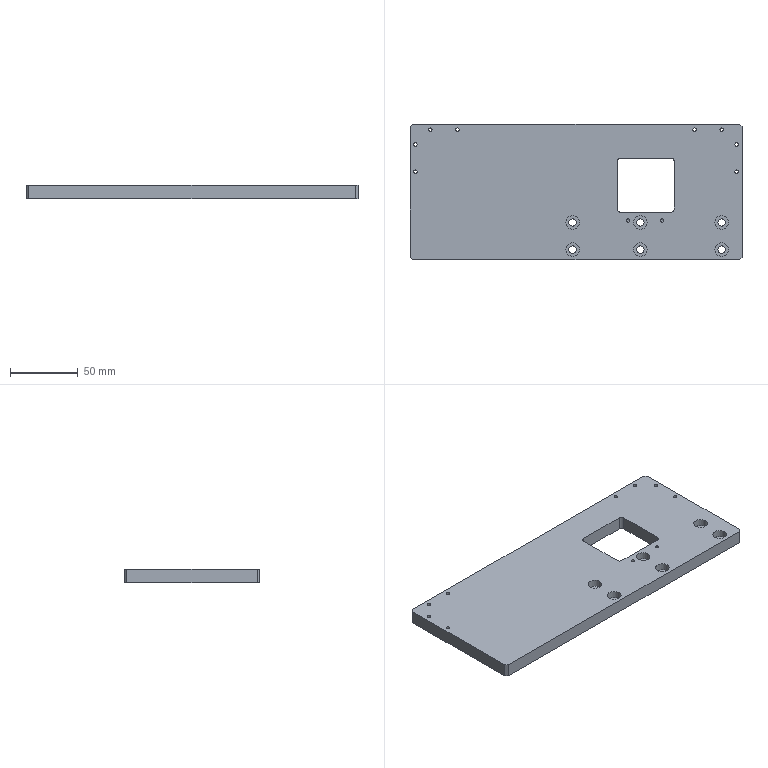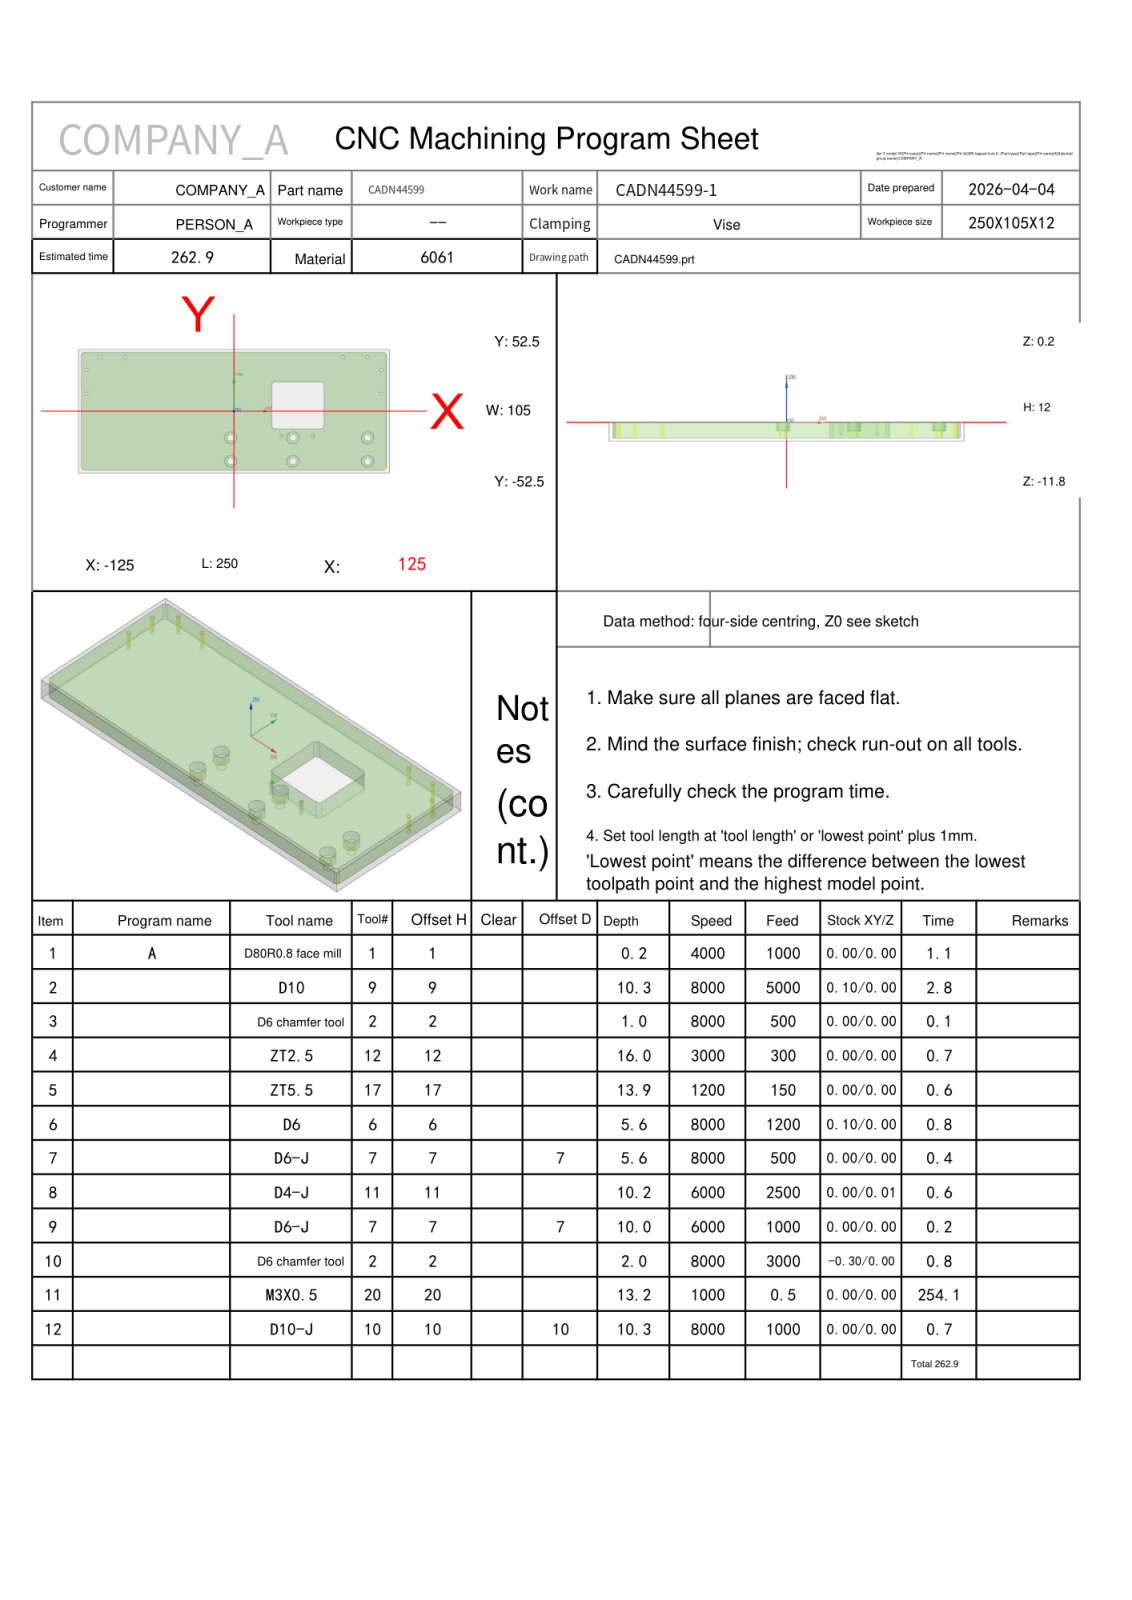NC program | NX | posted by the shop | part box 245 x 100 x 10 mm
Lines 755 to 1778 of 5259:
N8 T11 M06
(D4-J  D=4. R=0. H=11 ce=0.00 di=0.01)
G00 G90 G54 X33.121 Y-9.46 M03 S6000
G43 H11 Z20.
M08
Z.306
G01 X33.114 Y-9.461 Z.22 F2000.
X33.094 Y-9.463 Z.142
X33.064 Y-9.468 Z.072
X33.024 Y-9.475 Z.01
X32.977 Y-9.485 Z-.046
X32.925 Y-9.498 Z-.095
X32.868 Y-9.514 Z-.137
X32.811 Y-9.533 Z-.174
X32.753 Y-9.557 Z-.205
X32.696 Y-9.584 Z-.231
X32.644 Y-9.615 Z-.252
X32.597 Y-9.652 Z-.268
X32.557 Y-9.692 Z-.28
X32.527 Y-9.738 Z-.288
X32.507 Y-9.79 Z-.293
X32.5 Y-9.847 Z-.294
Y-12.565 F2500.
G03 X32.935 Y-13. I.435 J0.0
G01 X35.653
X35.696 Y-12.984 Z-.295
X35.718 Y-12.938 Z-.298
X35.72 Y-12.866 Z-.302
X35.703 Y-12.772 Z-.307
X35.67 Y-12.657 Z-.314
X35.622 Y-12.527 Z-.322
X35.56 Y-12.384 Z-.331
X35.486 Y-12.232 Z-.341
X35.402 Y-12.074 Z-.351
X35.309 Y-11.913 Z-.362
X35.209 Y-11.754 Z-.374
X34.969 Y-11.417 Z-.4
X34.704 Y-11.103 Z-.427
X34.413 Y-10.812 Z-.455
X34.098 Y-10.545 Z-.482
X33.76 Y-10.303 Z-.509
X33.599 Y-10.202 Z-.52
X33.437 Y-10.108 Z-.531
X33.278 Y-10.022 Z-.542
X33.124 Y-9.947 Z-.551
X32.979 Y-9.883 Z-.56
X32.847 Y-9.834 Z-.568
X32.731 Y-9.799 Z-.575
X32.635 Y-9.782 Z-.581
X32.563 Y-9.783 Z-.585
X32.516 Y-9.804 Z-.587
X32.5 Y-9.847 Z-.588
Y-12.565
G03 X32.935 Y-13. I.435 J0.0
G01 X35.653
X35.696 Y-12.984 Z-.589
X35.718 Y-12.938 Z-.592
X35.72 Y-12.866 Z-.596
X35.703 Y-12.772 Z-.601
X35.67 Y-12.657 Z-.608
X35.622 Y-12.527 Z-.616
X35.56 Y-12.384 Z-.625
X35.486 Y-12.232 Z-.635
X35.402 Y-12.074 Z-.645
X35.309 Y-11.913 Z-.656
X35.209 Y-11.754 Z-.668
X34.969 Y-11.417 Z-.694
X34.704 Y-11.103 Z-.722
X34.413 Y-10.812 Z-.749
X34.098 Y-10.545 Z-.776
X33.76 Y-10.303 Z-.803
X33.599 Y-10.202 Z-.814
X33.437 Y-10.108 Z-.825
X33.278 Y-10.022 Z-.836
X33.124 Y-9.947 Z-.846
X32.979 Y-9.883 Z-.855
X32.847 Y-9.834 Z-.862
X32.731 Y-9.799 Z-.869
X32.635 Y-9.782 Z-.875
X32.563 Y-9.783 Z-.879
X32.516 Y-9.804 Z-.881
X32.5 Y-9.847 Z-.882
Y-12.565
G03 X32.935 Y-13. I.435 J0.0
G01 X35.653
X35.696 Y-12.984 Z-.883
X35.718 Y-12.938 Z-.886
X35.72 Y-12.866 Z-.89
X35.703 Y-12.772 Z-.895
X35.67 Y-12.657 Z-.902
X35.622 Y-12.527 Z-.91
X35.56 Y-12.384 Z-.919
X35.486 Y-12.232 Z-.929
X35.402 Y-12.074 Z-.939
X35.309 Y-11.913 Z-.95
X35.209 Y-11.754 Z-.962
X34.969 Y-11.417 Z-.988
X34.704 Y-11.103 Z-1.016
X34.413 Y-10.812 Z-1.043
X34.098 Y-10.545 Z-1.07
X33.76 Y-10.303 Z-1.097
X33.599 Y-10.202 Z-1.108
X33.437 Y-10.108 Z-1.119
X33.278 Y-10.022 Z-1.13
X33.124 Y-9.947 Z-1.14
X32.979 Y-9.883 Z-1.149
X32.847 Y-9.834 Z-1.157
X32.731 Y-9.799 Z-1.163
X32.635 Y-9.782 Z-1.169
X32.563 Y-9.783 Z-1.173
X32.516 Y-9.804 Z-1.176
X32.5 Y-9.847
Y-12.565
G03 X32.935 Y-13. I.435 J0.0
G01 X35.653
X35.696 Y-12.984 Z-1.177
X35.718 Y-12.938 Z-1.18
X35.72 Y-12.866 Z-1.184
X35.703 Y-12.772 Z-1.19
X35.67 Y-12.657 Z-1.196
X35.622 Y-12.527 Z-1.204
X35.56 Y-12.384 Z-1.213
X35.486 Y-12.232 Z-1.223
X35.402 Y-12.074 Z-1.234
X35.309 Y-11.913 Z-1.245
X35.209 Y-11.754 Z-1.256
X34.969 Y-11.417 Z-1.283
X34.704 Y-11.103 Z-1.31
X34.413 Y-10.812 Z-1.337
X34.098 Y-10.545 Z-1.365
X33.76 Y-10.303 Z-1.391
X33.599 Y-10.202 Z-1.402
X33.437 Y-10.108 Z-1.414
X33.278 Y-10.022 Z-1.424
X33.124 Y-9.947 Z-1.434
X32.979 Y-9.883 Z-1.443
X32.847 Y-9.834 Z-1.451
X32.731 Y-9.799 Z-1.457
X32.635 Y-9.782 Z-1.463
X32.563 Y-9.783 Z-1.467
X32.516 Y-9.804 Z-1.47
X32.5 Y-9.847 Z-1.471
Y-12.565
G03 X32.935 Y-13. I.435 J0.0
G01 X35.653
X35.696 Y-12.984
X35.718 Y-12.938 Z-1.474
X35.72 Y-12.866 Z-1.478
X35.703 Y-12.772 Z-1.484
X35.67 Y-12.657 Z-1.49
X35.622 Y-12.527 Z-1.498
X35.56 Y-12.384 Z-1.507
X35.486 Y-12.232 Z-1.517
X35.402 Y-12.074 Z-1.528
X35.309 Y-11.913 Z-1.539
X35.209 Y-11.754 Z-1.55
X34.969 Y-11.417 Z-1.577
X34.704 Y-11.103 Z-1.604
X34.413 Y-10.812 Z-1.631
X34.098 Y-10.545 Z-1.659
X33.76 Y-10.303 Z-1.685
X33.599 Y-10.202 Z-1.697
X33.437 Y-10.108 Z-1.708
X33.278 Y-10.022 Z-1.718
X33.124 Y-9.947 Z-1.728
X32.979 Y-9.883 Z-1.737
X32.847 Y-9.834 Z-1.745
X32.731 Y-9.799 Z-1.752
X32.635 Y-9.782 Z-1.757
X32.563 Y-9.783 Z-1.761
X32.516 Y-9.804 Z-1.764
X32.5 Y-9.847 Z-1.765
Y-12.565
G03 X32.935 Y-13. I.435 J0.0
G01 X35.653
X35.696 Y-12.984 Z-1.766
X35.718 Y-12.938 Z-1.768
X35.72 Y-12.866 Z-1.772
X35.703 Y-12.772 Z-1.778
X35.67 Y-12.657 Z-1.785
X35.622 Y-12.527 Z-1.793
X35.56 Y-12.384 Z-1.801
X35.486 Y-12.232 Z-1.811
X35.402 Y-12.074 Z-1.822
X35.309 Y-11.913 Z-1.833
X35.209 Y-11.754 Z-1.844
X34.969 Y-11.417 Z-1.871
X34.704 Y-11.103 Z-1.898
X34.413 Y-10.812 Z-1.926
X34.098 Y-10.545 Z-1.953
X33.76 Y-10.303 Z-1.979
X33.599 Y-10.202 Z-1.991
X33.437 Y-10.108 Z-2.002
X33.278 Y-10.022 Z-2.012
X33.124 Y-9.947 Z-2.022
X32.979 Y-9.883 Z-2.031
X32.847 Y-9.834 Z-2.039
X32.731 Y-9.799 Z-2.046
X32.635 Y-9.782 Z-2.051
X32.563 Y-9.783 Z-2.055
X32.516 Y-9.804 Z-2.058
X32.5 Y-9.847 Z-2.059
Y-12.565
G03 X32.935 Y-13. I.435 J0.0
G01 X35.653
X35.696 Y-12.984 Z-2.06
X35.718 Y-12.938 Z-2.062
X35.72 Y-12.866 Z-2.066
X35.703 Y-12.772 Z-2.072
X35.67 Y-12.657 Z-2.079
X35.622 Y-12.527 Z-2.087
X35.56 Y-12.384 Z-2.096
X35.486 Y-12.232 Z-2.105
X35.402 Y-12.074 Z-2.116
X35.309 Y-11.913 Z-2.127
X35.209 Y-11.754 Z-2.138
X34.969 Y-11.417 Z-2.165
X34.704 Y-11.103 Z-2.192
X34.413 Y-10.812 Z-2.22
X34.098 Y-10.545 Z-2.247
X33.76 Y-10.303 Z-2.273
X33.599 Y-10.202 Z-2.285
X33.437 Y-10.108 Z-2.296
X33.278 Y-10.022 Z-2.306
X33.124 Y-9.947 Z-2.316
X32.979 Y-9.883 Z-2.325
X32.847 Y-9.834 Z-2.333
X32.731 Y-9.799 Z-2.34
X32.635 Y-9.782 Z-2.345
X32.563 Y-9.783 Z-2.349
X32.516 Y-9.804 Z-2.352
X32.5 Y-9.847 Z-2.353
Y-12.565
G03 X32.935 Y-13. I.435 J0.0
G01 X35.653
X35.696 Y-12.984 Z-2.354
X35.718 Y-12.938 Z-2.356
X35.72 Y-12.866 Z-2.361
X35.703 Y-12.772 Z-2.366
X35.67 Y-12.657 Z-2.373
X35.622 Y-12.527 Z-2.381
X35.56 Y-12.384 Z-2.39
X35.486 Y-12.232 Z-2.399
X35.402 Y-12.074 Z-2.41
X35.309 Y-11.913 Z-2.421
X35.209 Y-11.754 Z-2.433
X34.969 Y-11.417 Z-2.459
X34.704 Y-11.103 Z-2.486
X34.413 Y-10.812 Z-2.514
X34.098 Y-10.545 Z-2.541
X33.76 Y-10.303 Z-2.567
X33.599 Y-10.202 Z-2.579
X33.437 Y-10.108 Z-2.59
X33.278 Y-10.022 Z-2.601
X33.124 Y-9.947 Z-2.61
X32.979 Y-9.883 Z-2.619
X32.847 Y-9.834 Z-2.627
X32.731 Y-9.799 Z-2.634
X32.635 Y-9.782 Z-2.639
X32.563 Y-9.783 Z-2.644
X32.516 Y-9.804 Z-2.646
X32.5 Y-9.847 Z-2.647
Y-12.565
G03 X32.935 Y-13. I.435 J0.0
G01 X35.653
X35.696 Y-12.984 Z-2.648
X35.718 Y-12.938 Z-2.651
X35.72 Y-12.866 Z-2.655
X35.703 Y-12.772 Z-2.66
X35.67 Y-12.657 Z-2.667
X35.622 Y-12.527 Z-2.675
X35.56 Y-12.384 Z-2.684
X35.486 Y-12.232 Z-2.694
X35.402 Y-12.074 Z-2.704
X35.309 Y-11.913 Z-2.715
X35.209 Y-11.754 Z-2.727
X34.969 Y-11.417 Z-2.753
X34.704 Y-11.103 Z-2.78
X34.413 Y-10.812 Z-2.808
X34.098 Y-10.545 Z-2.835
X33.76 Y-10.303 Z-2.862
X33.599 Y-10.202 Z-2.873
X33.437 Y-10.108 Z-2.884
X33.278 Y-10.022 Z-2.895
X33.124 Y-9.947 Z-2.904
X32.979 Y-9.883 Z-2.913
X32.847 Y-9.834 Z-2.921
X32.731 Y-9.799 Z-2.928
X32.635 Y-9.782 Z-2.934
X32.563 Y-9.783 Z-2.938
X32.516 Y-9.804 Z-2.94
X32.5 Y-9.847 Z-2.941
Y-12.565
G03 X32.935 Y-13. I.435 J0.0
G01 X35.653
X35.696 Y-12.984 Z-2.942
X35.718 Y-12.938 Z-2.945
X35.72 Y-12.866 Z-2.949
X35.703 Y-12.772 Z-2.954
X35.67 Y-12.657 Z-2.961
X35.622 Y-12.527 Z-2.969
X35.56 Y-12.384 Z-2.978
X35.486 Y-12.232 Z-2.988
X35.402 Y-12.074 Z-2.998
X35.309 Y-11.913 Z-3.009
X35.209 Y-11.754 Z-3.021
X34.969 Y-11.417 Z-3.047
X34.704 Y-11.103 Z-3.074
X34.413 Y-10.812 Z-3.102
X34.098 Y-10.545 Z-3.129
X33.76 Y-10.303 Z-3.156
X33.599 Y-10.202 Z-3.167
X33.437 Y-10.108 Z-3.178
X33.278 Y-10.022 Z-3.189
X33.124 Y-9.947 Z-3.199
X32.979 Y-9.883 Z-3.207
X32.847 Y-9.834 Z-3.215
X32.731 Y-9.799 Z-3.222
X32.635 Y-9.782 Z-3.228
X32.563 Y-9.783 Z-3.232
X32.516 Y-9.804 Z-3.234
X32.5 Y-9.847 Z-3.235
Y-12.565
G03 X32.935 Y-13. I.435 J0.0
G01 X35.653
X35.696 Y-12.984 Z-3.236
X35.718 Y-12.938 Z-3.239
X35.72 Y-12.866 Z-3.243
X35.703 Y-12.772 Z-3.248
X35.67 Y-12.657 Z-3.255
X35.622 Y-12.527 Z-3.263
X35.56 Y-12.384 Z-3.272
X35.486 Y-12.232 Z-3.282
X35.402 Y-12.074 Z-3.292
X35.309 Y-11.913 Z-3.303
X35.209 Y-11.754 Z-3.315
X34.969 Y-11.417 Z-3.341
X34.704 Y-11.103 Z-3.369
X34.413 Y-10.812 Z-3.396
X34.098 Y-10.545 Z-3.423
X33.76 Y-10.303 Z-3.45
X33.599 Y-10.202 Z-3.461
X33.437 Y-10.108 Z-3.472
X33.278 Y-10.022 Z-3.483
X33.124 Y-9.947 Z-3.493
X32.979 Y-9.883 Z-3.502
X32.847 Y-9.834 Z-3.51
X32.731 Y-9.799 Z-3.516
X32.635 Y-9.782 Z-3.522
X32.563 Y-9.783 Z-3.526
X32.516 Y-9.804 Z-3.529
X32.5 Y-9.847
Y-12.565
G03 X32.935 Y-13. I.435 J0.0
G01 X35.653
X35.696 Y-12.984 Z-3.53
X35.718 Y-12.938 Z-3.533
X35.72 Y-12.866 Z-3.537
X35.703 Y-12.772 Z-3.543
X35.67 Y-12.657 Z-3.549
X35.622 Y-12.527 Z-3.557
X35.56 Y-12.384 Z-3.566
X35.486 Y-12.232 Z-3.576
X35.402 Y-12.074 Z-3.586
X35.309 Y-11.913 Z-3.598
X35.209 Y-11.754 Z-3.609
X34.969 Y-11.417 Z-3.635
X34.704 Y-11.103 Z-3.663
X34.413 Y-10.812 Z-3.69
X34.098 Y-10.545 Z-3.718
X33.76 Y-10.303 Z-3.744
X33.599 Y-10.202 Z-3.755
X33.437 Y-10.108 Z-3.766
X33.278 Y-10.022 Z-3.777
X33.124 Y-9.947 Z-3.787
X32.979 Y-9.883 Z-3.796
X32.847 Y-9.834 Z-3.804
X32.731 Y-9.799 Z-3.81
X32.635 Y-9.782 Z-3.816
X32.563 Y-9.783 Z-3.82
X32.516 Y-9.804 Z-3.823
X32.5 Y-9.847 Z-3.824
Y-12.565
G03 X32.935 Y-13. I.435 J0.0
G01 X35.653
X35.696 Y-12.984
X35.718 Y-12.938 Z-3.827
X35.72 Y-12.866 Z-3.831
X35.703 Y-12.772 Z-3.837
X35.67 Y-12.657 Z-3.843
X35.622 Y-12.527 Z-3.851
X35.56 Y-12.384 Z-3.86
X35.486 Y-12.232 Z-3.87
X35.402 Y-12.074 Z-3.881
X35.309 Y-11.913 Z-3.892
X35.209 Y-11.754 Z-3.903
X34.969 Y-11.417 Z-3.93
X34.704 Y-11.103 Z-3.957
X34.413 Y-10.812 Z-3.984
X34.098 Y-10.545 Z-4.012
X33.76 Y-10.303 Z-4.038
X33.599 Y-10.202 Z-4.05
X33.437 Y-10.108 Z-4.061
X33.278 Y-10.022 Z-4.071
X33.124 Y-9.947 Z-4.081
X32.979 Y-9.883 Z-4.09
X32.847 Y-9.834 Z-4.098
X32.731 Y-9.799 Z-4.105
X32.635 Y-9.782 Z-4.11
X32.563 Y-9.783 Z-4.114
X32.516 Y-9.804 Z-4.117
X32.5 Y-9.847 Z-4.118
Y-12.565
G03 X32.935 Y-13. I.435 J0.0
G01 X35.653
X35.696 Y-12.984 Z-4.119
X35.718 Y-12.938 Z-4.121
X35.72 Y-12.866 Z-4.125
X35.703 Y-12.772 Z-4.131
X35.67 Y-12.657 Z-4.138
X35.622 Y-12.527 Z-4.145
X35.56 Y-12.384 Z-4.154
X35.486 Y-12.232 Z-4.164
X35.402 Y-12.074 Z-4.175
X35.309 Y-11.913 Z-4.186
X35.209 Y-11.754 Z-4.197
X34.969 Y-11.417 Z-4.224
X34.704 Y-11.103 Z-4.251
X34.413 Y-10.812 Z-4.278
X34.098 Y-10.545 Z-4.306
X33.76 Y-10.303 Z-4.332
X33.599 Y-10.202 Z-4.344
X33.437 Y-10.108 Z-4.355
X33.278 Y-10.022 Z-4.365
X33.124 Y-9.947 Z-4.375
X32.979 Y-9.883 Z-4.384
X32.847 Y-9.834 Z-4.392
X32.731 Y-9.799 Z-4.399
X32.635 Y-9.782 Z-4.404
X32.563 Y-9.783 Z-4.408
X32.516 Y-9.804 Z-4.411
X32.5 Y-9.847 Z-4.412
Y-12.565
G03 X32.935 Y-13. I.435 J0.0
G01 X35.653
X35.696 Y-12.984 Z-4.413
X35.718 Y-12.938 Z-4.415
X35.72 Y-12.866 Z-4.419
X35.703 Y-12.772 Z-4.425
X35.67 Y-12.657 Z-4.432
X35.622 Y-12.527 Z-4.44
X35.56 Y-12.384 Z-4.449
X35.486 Y-12.232 Z-4.458
X35.402 Y-12.074 Z-4.469
X35.309 Y-11.913 Z-4.48
X35.209 Y-11.754 Z-4.491
X34.969 Y-11.417 Z-4.518
X34.704 Y-11.103 Z-4.545
X34.413 Y-10.812 Z-4.573
X34.098 Y-10.545 Z-4.6
X33.76 Y-10.303 Z-4.626
X33.599 Y-10.202 Z-4.638
X33.437 Y-10.108 Z-4.649
X33.278 Y-10.022 Z-4.659
X33.124 Y-9.947 Z-4.669
X32.979 Y-9.883 Z-4.678
X32.847 Y-9.834 Z-4.686
X32.731 Y-9.799 Z-4.693
X32.635 Y-9.782 Z-4.698
X32.563 Y-9.783 Z-4.702
X32.516 Y-9.804 Z-4.705
X32.5 Y-9.847 Z-4.706
Y-12.565
G03 X32.935 Y-13. I.435 J0.0
G01 X35.653
X35.696 Y-12.984 Z-4.707
X35.718 Y-12.938 Z-4.709
X35.72 Y-12.866 Z-4.713
X35.703 Y-12.772 Z-4.719
X35.67 Y-12.657 Z-4.726
X35.622 Y-12.527 Z-4.734
X35.56 Y-12.384 Z-4.743
X35.486 Y-12.232 Z-4.752
X35.402 Y-12.074 Z-4.763
X35.309 Y-11.913 Z-4.774
X35.209 Y-11.754 Z-4.786
X34.969 Y-11.417 Z-4.812
X34.704 Y-11.103 Z-4.839
X34.413 Y-10.812 Z-4.867
X34.098 Y-10.545 Z-4.894
X33.76 Y-10.303 Z-4.92
X33.599 Y-10.202 Z-4.932
X33.437 Y-10.108 Z-4.943
X33.278 Y-10.022 Z-4.953
X33.124 Y-9.947 Z-4.963
X32.979 Y-9.883 Z-4.972
X32.847 Y-9.834 Z-4.98
X32.731 Y-9.799 Z-4.987
X32.635 Y-9.782 Z-4.992
X32.563 Y-9.783 Z-4.997
X32.516 Y-9.804 Z-4.999
X32.5 Y-9.847 Z-5.
Y-12.565
G03 X32.935 Y-13. I.435 J0.0
G01 X35.653
X35.696 Y-12.984 Z-5.001
X35.718 Y-12.938 Z-5.003
X35.72 Y-12.866 Z-5.008
X35.703 Y-12.772 Z-5.013
X35.67 Y-12.657 Z-5.02
X35.622 Y-12.527 Z-5.028
X35.56 Y-12.384 Z-5.037
X35.486 Y-12.232 Z-5.047
X35.402 Y-12.074 Z-5.057
X35.309 Y-11.913 Z-5.068
X35.209 Y-11.754 Z-5.08
X34.969 Y-11.417 Z-5.106
X34.704 Y-11.103 Z-5.133
X34.413 Y-10.812 Z-5.161
X34.098 Y-10.545 Z-5.188
X33.76 Y-10.303 Z-5.214
X33.599 Y-10.202 Z-5.226
X33.437 Y-10.108 Z-5.237
X33.278 Y-10.022 Z-5.248
X33.124 Y-9.947 Z-5.257
X32.979 Y-9.883 Z-5.266
X32.847 Y-9.834 Z-5.274
X32.731 Y-9.799 Z-5.281
X32.635 Y-9.782 Z-5.287
X32.563 Y-9.783 Z-5.291
X32.516 Y-9.804 Z-5.293
X32.5 Y-9.847 Z-5.294
Y-12.565
G03 X32.935 Y-13. I.435 J0.0
G01 X35.653
X35.696 Y-12.984 Z-5.295
X35.718 Y-12.938 Z-5.298
X35.72 Y-12.866 Z-5.302
X35.703 Y-12.772 Z-5.307
X35.67 Y-12.657 Z-5.314
X35.622 Y-12.527 Z-5.322
X35.56 Y-12.384 Z-5.331
X35.486 Y-12.232 Z-5.341
X35.402 Y-12.074 Z-5.351
X35.309 Y-11.913 Z-5.362
X35.209 Y-11.754 Z-5.374
X34.969 Y-11.417 Z-5.4
X34.704 Y-11.103 Z-5.427
X34.413 Y-10.812 Z-5.455
X34.098 Y-10.545 Z-5.482
X33.76 Y-10.303 Z-5.509
X33.599 Y-10.202 Z-5.52
X33.437 Y-10.108 Z-5.531
X33.278 Y-10.022 Z-5.542
X33.124 Y-9.947 Z-5.551
X32.979 Y-9.883 Z-5.56
X32.847 Y-9.834 Z-5.568
X32.731 Y-9.799 Z-5.575
X32.635 Y-9.782 Z-5.581
X32.563 Y-9.783 Z-5.585
X32.516 Y-9.804 Z-5.587
X32.5 Y-9.847 Z-5.588
Y-12.565
G03 X32.935 Y-13. I.435 J0.0
G01 X35.653
X35.696 Y-12.984 Z-5.589
X35.718 Y-12.938 Z-5.592
X35.72 Y-12.866 Z-5.596
X35.703 Y-12.772 Z-5.601
X35.67 Y-12.657 Z-5.608
X35.622 Y-12.527 Z-5.616
X35.56 Y-12.384 Z-5.625
X35.486 Y-12.232 Z-5.635
X35.402 Y-12.074 Z-5.645
X35.309 Y-11.913 Z-5.656
X35.209 Y-11.754 Z-5.668
X34.969 Y-11.417 Z-5.694
X34.704 Y-11.103 Z-5.722
X34.413 Y-10.812 Z-5.749
X34.098 Y-10.545 Z-5.776
X33.76 Y-10.303 Z-5.803
X33.599 Y-10.202 Z-5.814
X33.437 Y-10.108 Z-5.825
X33.278 Y-10.022 Z-5.836
X33.124 Y-9.947 Z-5.846
X32.979 Y-9.883 Z-5.855
X32.847 Y-9.834 Z-5.862
X32.731 Y-9.799 Z-5.869
X32.635 Y-9.782 Z-5.875
X32.563 Y-9.783 Z-5.879
X32.516 Y-9.804 Z-5.881
X32.5 Y-9.847 Z-5.882
Y-12.565
G03 X32.935 Y-13. I.435 J0.0
G01 X35.653
X35.696 Y-12.984 Z-5.883
X35.718 Y-12.938 Z-5.886
X35.72 Y-12.866 Z-5.89
X35.703 Y-12.772 Z-5.895
X35.67 Y-12.657 Z-5.902
X35.622 Y-12.527 Z-5.91
X35.56 Y-12.384 Z-5.919
X35.486 Y-12.232 Z-5.929
X35.402 Y-12.074 Z-5.939
X35.309 Y-11.913 Z-5.95
X35.209 Y-11.754 Z-5.962
X34.969 Y-11.417 Z-5.988
X34.704 Y-11.103 Z-6.016
X34.413 Y-10.812 Z-6.043
X34.098 Y-10.545 Z-6.07
X33.76 Y-10.303 Z-6.097
X33.599 Y-10.202 Z-6.108
X33.437 Y-10.108 Z-6.119
X33.278 Y-10.022 Z-6.13
X33.124 Y-9.947 Z-6.14
X32.979 Y-9.883 Z-6.149
X32.847 Y-9.834 Z-6.157
X32.731 Y-9.799 Z-6.163
X32.635 Y-9.782 Z-6.169
X32.563 Y-9.783 Z-6.173
X32.516 Y-9.804 Z-6.176
X32.5 Y-9.847
Y-12.565
G03 X32.935 Y-13. I.435 J0.0
G01 X35.653
X35.696 Y-12.984 Z-6.177
X35.718 Y-12.938 Z-6.18
X35.72 Y-12.866 Z-6.184
X35.703 Y-12.772 Z-6.19
X35.67 Y-12.657 Z-6.196
X35.622 Y-12.527 Z-6.204
X35.56 Y-12.384 Z-6.213
X35.486 Y-12.232 Z-6.223
X35.402 Y-12.074 Z-6.234
X35.309 Y-11.913 Z-6.245
X35.209 Y-11.754 Z-6.256
X34.969 Y-11.417 Z-6.283
X34.704 Y-11.103 Z-6.31
X34.413 Y-10.812 Z-6.337
X34.098 Y-10.545 Z-6.365
X33.76 Y-10.303 Z-6.391
X33.599 Y-10.202 Z-6.402
X33.437 Y-10.108 Z-6.414
X33.278 Y-10.022 Z-6.424
X33.124 Y-9.947 Z-6.434
X32.979 Y-9.883 Z-6.443
X32.847 Y-9.834 Z-6.451
X32.731 Y-9.799 Z-6.457
X32.635 Y-9.782 Z-6.463
X32.563 Y-9.783 Z-6.467
X32.516 Y-9.804 Z-6.47
X32.5 Y-9.847 Z-6.471
Y-12.565
G03 X32.935 Y-13. I.435 J0.0
G01 X35.653
X35.696 Y-12.984
X35.718 Y-12.938 Z-6.474
X35.72 Y-12.866 Z-6.478
X35.703 Y-12.772 Z-6.484
X35.67 Y-12.657 Z-6.49
X35.622 Y-12.527 Z-6.498
X35.56 Y-12.384 Z-6.507
X35.486 Y-12.232 Z-6.517
X35.402 Y-12.074 Z-6.528
X35.309 Y-11.913 Z-6.539
X35.209 Y-11.754 Z-6.55
X34.969 Y-11.417 Z-6.577
X34.704 Y-11.103 Z-6.604
X34.413 Y-10.812 Z-6.631
X34.098 Y-10.545 Z-6.659
X33.76 Y-10.303 Z-6.685
X33.599 Y-10.202 Z-6.697
X33.437 Y-10.108 Z-6.708
X33.278 Y-10.022 Z-6.718
X33.124 Y-9.947 Z-6.728
X32.979 Y-9.883 Z-6.737
X32.847 Y-9.834 Z-6.745
X32.731 Y-9.799 Z-6.752
X32.635 Y-9.782 Z-6.757
X32.563 Y-9.783 Z-6.761
X32.516 Y-9.804 Z-6.764
X32.5 Y-9.847 Z-6.765
Y-12.565
G03 X32.935 Y-13. I.435 J0.0
G01 X35.653
X35.696 Y-12.984 Z-6.766
X35.718 Y-12.938 Z-6.768
X35.72 Y-12.866 Z-6.772
X35.703 Y-12.772 Z-6.778
X35.67 Y-12.657 Z-6.785
X35.622 Y-12.527 Z-6.793
X35.56 Y-12.384 Z-6.801
X35.486 Y-12.232 Z-6.811
X35.402 Y-12.074 Z-6.822
X35.309 Y-11.913 Z-6.833
X35.209 Y-11.754 Z-6.844
X34.969 Y-11.417 Z-6.871
X34.704 Y-11.103 Z-6.898
X34.413 Y-10.812 Z-6.926
X34.098 Y-10.545 Z-6.953
X33.76 Y-10.303 Z-6.979
X33.599 Y-10.202 Z-6.991
X33.437 Y-10.108 Z-7.002
X33.278 Y-10.022 Z-7.012
X33.124 Y-9.947 Z-7.022
X32.979 Y-9.883 Z-7.031
X32.847 Y-9.834 Z-7.039
X32.731 Y-9.799 Z-7.046
X32.635 Y-9.782 Z-7.051
X32.563 Y-9.783 Z-7.055
X32.516 Y-9.804 Z-7.058
X32.5 Y-9.847 Z-7.059
Y-12.565
G03 X32.935 Y-13. I.435 J0.0
G01 X35.653
X35.696 Y-12.984 Z-7.06
X35.718 Y-12.938 Z-7.062
X35.72 Y-12.866 Z-7.066
X35.703 Y-12.772 Z-7.072
X35.67 Y-12.657 Z-7.079
X35.622 Y-12.527 Z-7.087
X35.56 Y-12.384 Z-7.096
X35.486 Y-12.232 Z-7.105
X35.402 Y-12.074 Z-7.116
X35.309 Y-11.913 Z-7.127
X35.209 Y-11.754 Z-7.138
X34.969 Y-11.417 Z-7.165
X34.704 Y-11.103 Z-7.192
X34.413 Y-10.812 Z-7.22
X34.098 Y-10.545 Z-7.247
X33.76 Y-10.303 Z-7.273
X33.599 Y-10.202 Z-7.285
X33.437 Y-10.108 Z-7.296
X33.278 Y-10.022 Z-7.306
X33.124 Y-9.947 Z-7.316
X32.979 Y-9.883 Z-7.325
X32.847 Y-9.834 Z-7.333
X32.731 Y-9.799 Z-7.34
X32.635 Y-9.782 Z-7.345
X32.563 Y-9.783 Z-7.349
X32.516 Y-9.804 Z-7.352
X32.5 Y-9.847 Z-7.353
Y-12.565
G03 X32.935 Y-13. I.435 J0.0
G01 X35.653
X35.696 Y-12.984 Z-7.354
X35.718 Y-12.938 Z-7.356
X35.72 Y-12.866 Z-7.361
X35.703 Y-12.772 Z-7.366
X35.67 Y-12.657 Z-7.373
X35.622 Y-12.527 Z-7.381
X35.56 Y-12.384 Z-7.39
X35.486 Y-12.232 Z-7.399
X35.402 Y-12.074 Z-7.41
X35.309 Y-11.913 Z-7.421
X35.209 Y-11.754 Z-7.433
X34.969 Y-11.417 Z-7.459
X34.704 Y-11.103 Z-7.486
X34.413 Y-10.812 Z-7.514
X34.098 Y-10.545 Z-7.541
X33.76 Y-10.303 Z-7.567
X33.599 Y-10.202 Z-7.579
X33.437 Y-10.108 Z-7.59
X33.278 Y-10.022 Z-7.601
X33.124 Y-9.947 Z-7.61
X32.979 Y-9.883 Z-7.619
X32.847 Y-9.834 Z-7.627
X32.731 Y-9.799 Z-7.634
X32.635 Y-9.782 Z-7.639
X32.563 Y-9.783 Z-7.644
X32.516 Y-9.804 Z-7.646
X32.5 Y-9.847 Z-7.647
Y-12.565
G03 X32.935 Y-13. I.435 J0.0
G01 X35.653
X35.696 Y-12.984 Z-7.648
X35.718 Y-12.938 Z-7.651
X35.72 Y-12.866 Z-7.655
X35.703 Y-12.772 Z-7.66
X35.67 Y-12.657 Z-7.667
X35.622 Y-12.527 Z-7.675
X35.56 Y-12.384 Z-7.684
X35.486 Y-12.232 Z-7.694
X35.402 Y-12.074 Z-7.704
X35.309 Y-11.913 Z-7.715
X35.209 Y-11.754 Z-7.727
X34.969 Y-11.417 Z-7.753
X34.704 Y-11.103 Z-7.78
X34.413 Y-10.812 Z-7.808
X34.098 Y-10.545 Z-7.835
X33.76 Y-10.303 Z-7.862
X33.599 Y-10.202 Z-7.873
X33.437 Y-10.108 Z-7.884
X33.278 Y-10.022 Z-7.895
X33.124 Y-9.947 Z-7.904
X32.979 Y-9.883 Z-7.913
X32.847 Y-9.834 Z-7.921
X32.731 Y-9.799 Z-7.928
X32.635 Y-9.782 Z-7.934
X32.563 Y-9.783 Z-7.938
X32.516 Y-9.804 Z-7.94
X32.5 Y-9.847 Z-7.941
Y-12.565
G03 X32.935 Y-13. I.435 J0.0
G01 X35.653
X35.696 Y-12.984 Z-7.942
X35.718 Y-12.938 Z-7.945
X35.72 Y-12.866 Z-7.949
X35.703 Y-12.772 Z-7.954
X35.67 Y-12.657 Z-7.961
X35.622 Y-12.527 Z-7.969
X35.56 Y-12.384 Z-7.978
X35.486 Y-12.232 Z-7.988
X35.402 Y-12.074 Z-7.998
X35.309 Y-11.913 Z-8.009
X35.209 Y-11.754 Z-8.021
X34.969 Y-11.417 Z-8.047
X34.704 Y-11.103 Z-8.074
X34.413 Y-10.812 Z-8.102
X34.098 Y-10.545 Z-8.129
X33.76 Y-10.303 Z-8.156
X33.599 Y-10.202 Z-8.167
X33.437 Y-10.108 Z-8.178
X33.278 Y-10.022 Z-8.189
X33.124 Y-9.947 Z-8.199
X32.979 Y-9.883 Z-8.207
X32.847 Y-9.834 Z-8.215
X32.731 Y-9.799 Z-8.222
X32.635 Y-9.782 Z-8.228
X32.563 Y-9.783 Z-8.232
X32.516 Y-9.804 Z-8.234
X32.5 Y-9.847 Z-8.235
Y-12.565
G03 X32.935 Y-13. I.435 J0.0
G01 X35.653
X35.696 Y-12.984 Z-8.236
X35.718 Y-12.938 Z-8.239
X35.72 Y-12.866 Z-8.243
X35.703 Y-12.772 Z-8.248
X35.67 Y-12.657 Z-8.255
X35.622 Y-12.527 Z-8.263
X35.56 Y-12.384 Z-8.272
X35.486 Y-12.232 Z-8.282
X35.402 Y-12.074 Z-8.292
X35.309 Y-11.913 Z-8.303
X35.209 Y-11.754 Z-8.315
X34.969 Y-11.417 Z-8.341
X34.704 Y-11.103 Z-8.369
X34.413 Y-10.812 Z-8.396
X34.098 Y-10.545 Z-8.423
X33.76 Y-10.303 Z-8.45
X33.599 Y-10.202 Z-8.461
X33.437 Y-10.108 Z-8.472
X33.278 Y-10.022 Z-8.483
X33.124 Y-9.947 Z-8.493
X32.979 Y-9.883 Z-8.502
X32.847 Y-9.834 Z-8.51
X32.731 Y-9.799 Z-8.516
X32.635 Y-9.782 Z-8.522
X32.563 Y-9.783 Z-8.526
X32.516 Y-9.804 Z-8.529
X32.5 Y-9.847
Y-12.565
G03 X32.935 Y-13. I.435 J0.0
G01 X35.653
X35.696 Y-12.984 Z-8.53
X35.718 Y-12.938 Z-8.533
X35.72 Y-12.866 Z-8.537
X35.703 Y-12.772 Z-8.543
X35.67 Y-12.657 Z-8.549
X35.622 Y-12.527 Z-8.557
X35.56 Y-12.384 Z-8.566
X35.486 Y-12.232 Z-8.576
X35.402 Y-12.074 Z-8.586
X35.309 Y-11.913 Z-8.598
X35.209 Y-11.754 Z-8.609
X34.969 Y-11.417 Z-8.635
X34.704 Y-11.103 Z-8.663
X34.413 Y-10.812 Z-8.69
X34.098 Y-10.545 Z-8.718
X33.76 Y-10.303 Z-8.744
X33.599 Y-10.202 Z-8.755
X33.437 Y-10.108 Z-8.766
X33.278 Y-10.022 Z-8.777
X33.124 Y-9.947 Z-8.787
X32.979 Y-9.883 Z-8.796
X32.847 Y-9.834 Z-8.804
X32.731 Y-9.799 Z-8.81
X32.635 Y-9.782 Z-8.816
X32.563 Y-9.783 Z-8.82
X32.516 Y-9.804 Z-8.823
X32.5 Y-9.847 Z-8.824
Y-12.565
G03 X32.935 Y-13. I.435 J0.0
G01 X35.653
X35.696 Y-12.984
X35.718 Y-12.938 Z-8.827
X35.72 Y-12.866 Z-8.831
X35.703 Y-12.772 Z-8.837
X35.67 Y-12.657 Z-8.843
X35.622 Y-12.527 Z-8.851
X35.56 Y-12.384 Z-8.86
X35.486 Y-12.232 Z-8.87
X35.402 Y-12.074 Z-8.881
X35.309 Y-11.913 Z-8.892
X35.209 Y-11.754 Z-8.903
X34.969 Y-11.417 Z-8.93
X34.704 Y-11.103 Z-8.957
X34.413 Y-10.812 Z-8.984
X34.098 Y-10.545 Z-9.012
X33.76 Y-10.303 Z-9.038
X33.599 Y-10.202 Z-9.05
X33.437 Y-10.108 Z-9.061
X33.278 Y-10.022 Z-9.071
X33.124 Y-9.947 Z-9.081
X32.979 Y-9.883 Z-9.09
X32.847 Y-9.834 Z-9.098
X32.731 Y-9.799 Z-9.105
X32.635 Y-9.782 Z-9.11
X32.563 Y-9.783 Z-9.114
X32.516 Y-9.804 Z-9.117
X32.5 Y-9.847 Z-9.118
Y-12.565
G03 X32.935 Y-13. I.435 J0.0
G01 X35.653
X35.696 Y-12.984 Z-9.119
X35.718 Y-12.938 Z-9.121
X35.72 Y-12.866 Z-9.125
X35.703 Y-12.772 Z-9.131
X35.67 Y-12.657 Z-9.138
X35.622 Y-12.527 Z-9.145
X35.56 Y-12.384 Z-9.154
X35.486 Y-12.232 Z-9.164
X35.402 Y-12.074 Z-9.175
X35.309 Y-11.913 Z-9.186
X35.209 Y-11.754 Z-9.197
X34.969 Y-11.417 Z-9.224
X34.704 Y-11.103 Z-9.251
X34.413 Y-10.812 Z-9.278
X34.098 Y-10.545 Z-9.306
X33.76 Y-10.303 Z-9.332
X33.599 Y-10.202 Z-9.344
X33.437 Y-10.108 Z-9.355
X33.278 Y-10.022 Z-9.365
X33.124 Y-9.947 Z-9.375
X32.979 Y-9.883 Z-9.384
X32.847 Y-9.834 Z-9.392
X32.731 Y-9.799 Z-9.399
X32.635 Y-9.782 Z-9.404
X32.563 Y-9.783 Z-9.408
X32.516 Y-9.804 Z-9.411
X32.5 Y-9.847 Z-9.412
Y-12.565
G03 X32.935 Y-13. I.435 J0.0
G01 X35.653
X35.696 Y-12.984 Z-9.413
X35.718 Y-12.938 Z-9.415
X35.72 Y-12.866 Z-9.419
X35.703 Y-12.772 Z-9.425
X35.67 Y-12.657 Z-9.432
X35.622 Y-12.527 Z-9.44
X35.56 Y-12.384 Z-9.449
X35.486 Y-12.232 Z-9.458
X35.402 Y-12.074 Z-9.469
X35.309 Y-11.913 Z-9.48
X35.209 Y-11.754 Z-9.491
X34.969 Y-11.417 Z-9.518
X34.704 Y-11.103 Z-9.545
X34.413 Y-10.812 Z-9.573
X34.098 Y-10.545 Z-9.6
X33.76 Y-10.303 Z-9.626
X33.599 Y-10.202 Z-9.638
X33.437 Y-10.108 Z-9.649
X33.278 Y-10.022 Z-9.659
X33.124 Y-9.947 Z-9.669
X32.979 Y-9.883 Z-9.678
X32.847 Y-9.834 Z-9.686
X32.731 Y-9.799 Z-9.693
X32.635 Y-9.782 Z-9.698
X32.563 Y-9.783 Z-9.702
X32.516 Y-9.804 Z-9.705
X32.5 Y-9.847 Z-9.706
Y-12.565
G03 X32.935 Y-13. I.435 J0.0
G01 X35.653
X35.696 Y-12.984 Z-9.707
X35.718 Y-12.938 Z-9.709
X35.72 Y-12.866 Z-9.713
X35.703 Y-12.772 Z-9.719
X35.67 Y-12.657 Z-9.726
X35.622 Y-12.527 Z-9.734
X35.56 Y-12.384 Z-9.743
X35.486 Y-12.232 Z-9.752
X35.402 Y-12.074 Z-9.763
X35.309 Y-11.913 Z-9.774
X35.209 Y-11.754 Z-9.786
X34.969 Y-11.417 Z-9.812
X34.704 Y-11.103 Z-9.839
X34.413 Y-10.812 Z-9.867
X34.098 Y-10.545 Z-9.894
X33.76 Y-10.303 Z-9.92
X33.599 Y-10.202 Z-9.932
X33.437 Y-10.108 Z-9.943
X33.278 Y-10.022 Z-9.953
X33.124 Y-9.947 Z-9.963
X32.979 Y-9.883 Z-9.972
X32.847 Y-9.834 Z-9.98
X32.731 Y-9.799 Z-9.987
X32.635 Y-9.782 Z-9.992
X32.563 Y-9.783 Z-9.997
X32.516 Y-9.804 Z-9.999
X32.5 Y-9.847 Z-10.
Y-12.565
G03 X32.935 Y-13. I.435 J0.0
G01 X35.653
X35.71 Y-12.993 Z-9.999
X35.762 Y-12.974 Z-9.994
X35.809 Y-12.945 Z-9.986
X35.851 Y-12.906 Z-9.974
X35.888 Y-12.861 Z-9.958
X35.92 Y-12.81 Z-9.937
X35.949 Y-12.756 Z-9.911
X35.973 Y-12.7 Z-9.88
X35.994 Y-12.644 Z-9.843